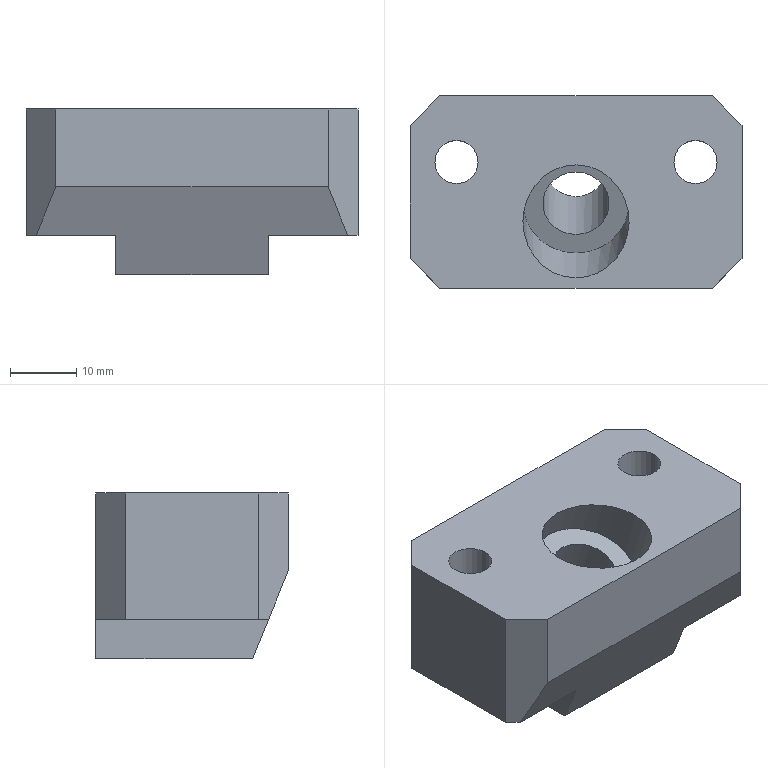Part | STEP file | lll_id298_x_t | 1 solid | 24 faces | box 50 x 29 x 25 mm | volume 24612 mm3 | plane 18 | cylinder 6 | commonest cylinder face diameters 6.5 x2 11 x2 10 x1 16 x1
STEP:
#1=CARTESIAN_POINT('',(0.,114.845,5.));
#2=VERTEX_POINT('',#1);
#3=CARTESIAN_POINT('',(0.,120.165,5.));
#4=DIRECTION('',(0.,0.,-1.));
#5=DIRECTION('',(0.,-1.,0.));
#6=AXIS2_PLACEMENT_3D('',#3,#4,#5);
#7=ELLIPSE('',#6,5.321,5.);
#8=EDGE_CURVE('',#2,#2,#7,.T.);
#9=ORIENTED_EDGE('',*,*,#8,.F.);
#10=EDGE_LOOP('',(#9));
#11=FACE_BOUND('',#10,.T.);
#12=CARTESIAN_POINT('',(-11.5,106.372,5.));
#13=VERTEX_POINT('',#12);
#14=CARTESIAN_POINT('',(11.5,106.372,5.));
#15=VERTEX_POINT('',#14);
#16=CARTESIAN_POINT('',(0.,106.372,5.));
#17=DIRECTION('',(1.,0.,0.));
#18=VECTOR('',#17,1.);
#19=LINE('',#16,#18);
#20=EDGE_CURVE('',#13,#15,#19,.T.);
#21=ORIENTED_EDGE('',*,*,#20,.F.);
#22=CARTESIAN_POINT('',(-11.5,130.,5.));
#23=VERTEX_POINT('',#22);
#24=CARTESIAN_POINT('',(-11.5,117.583,5.));
#25=DIRECTION('',(0.,-1.,0.));
#26=VECTOR('',#25,1.);
#27=LINE('',#24,#26);
#28=EDGE_CURVE('',#23,#13,#27,.T.);
#29=ORIENTED_EDGE('',*,*,#28,.F.);
#30=CARTESIAN_POINT('',(11.5,130.,5.));
#31=VERTEX_POINT('',#30);
#32=CARTESIAN_POINT('',(0.,130.,5.));
#33=DIRECTION('',(1.,0.,0.));
#34=VECTOR('',#33,1.);
#35=LINE('',#32,#34);
#36=EDGE_CURVE('',#23,#31,#35,.T.);
#37=ORIENTED_EDGE('',*,*,#36,.T.);
#38=CARTESIAN_POINT('',(11.5,117.583,5.));
#39=DIRECTION('',(0.,-1.,0.));
#40=VECTOR('',#39,1.);
#41=LINE('',#38,#40);
#42=EDGE_CURVE('',#31,#15,#41,.T.);
#43=ORIENTED_EDGE('',*,*,#42,.T.);
#44=EDGE_LOOP('',(#21,#29,#37,#43));
#45=FACE_BOUND('',#44,.T.);
#46=CARTESIAN_POINT('',(0.,116.372,5.));
#47=DIRECTION('',(0.,0.,-1.));
#48=DIRECTION('',(1.,0.,0.));
#49=AXIS2_PLACEMENT_3D('',#46,#47,#48);
#50=PLANE('',#49);
#51=ADVANCED_FACE('',(#11,#45),#50,.T.);
#52=CARTESIAN_POINT('',(-20.5,130.,11.));
#53=VERTEX_POINT('',#52);
#54=CARTESIAN_POINT('',(-11.5,130.,11.));
#55=VERTEX_POINT('',#54);
#56=CARTESIAN_POINT('',(0.,130.,11.));
#57=DIRECTION('',(1.,0.,0.));
#58=VECTOR('',#57,1.);
#59=LINE('',#56,#58);
#60=EDGE_CURVE('',#53,#55,#59,.T.);
#61=ORIENTED_EDGE('',*,*,#60,.F.);
#62=CARTESIAN_POINT('',(-20.5,130.,30.));
#63=VERTEX_POINT('',#62);
#64=CARTESIAN_POINT('',(-20.5,130.,-70.5));
#65=DIRECTION('',(0.,0.,1.));
#66=VECTOR('',#65,1.);
#67=LINE('',#64,#66);
#68=EDGE_CURVE('',#53,#63,#67,.T.);
#69=ORIENTED_EDGE('',*,*,#68,.T.);
#70=CARTESIAN_POINT('',(20.5,130.,30.));
#71=VERTEX_POINT('',#70);
#72=CARTESIAN_POINT('',(-0.004167,130.,30.));
#73=DIRECTION('',(1.,0.,0.));
#74=VECTOR('',#73,1.);
#75=LINE('',#72,#74);
#76=EDGE_CURVE('',#63,#71,#75,.T.);
#77=ORIENTED_EDGE('',*,*,#76,.T.);
#78=CARTESIAN_POINT('',(20.5,130.,11.));
#79=VERTEX_POINT('',#78);
#80=CARTESIAN_POINT('',(20.5,130.,11.));
#81=DIRECTION('',(0.,0.,-1.));
#82=VECTOR('',#81,1.);
#83=LINE('',#80,#82);
#84=EDGE_CURVE('',#71,#79,#83,.T.);
#85=ORIENTED_EDGE('',*,*,#84,.T.);
#86=CARTESIAN_POINT('',(11.5,130.,11.));
#87=VERTEX_POINT('',#86);
#88=CARTESIAN_POINT('',(0.,130.,11.));
#89=DIRECTION('',(1.,0.,0.));
#90=VECTOR('',#89,1.);
#91=LINE('',#88,#90);
#92=EDGE_CURVE('',#87,#79,#91,.T.);
#93=ORIENTED_EDGE('',*,*,#92,.F.);
#94=CARTESIAN_POINT('',(11.5,130.,2.003));
#95=DIRECTION('',(0.,0.,-1.));
#96=VECTOR('',#95,1.);
#97=LINE('',#94,#96);
#98=EDGE_CURVE('',#87,#31,#97,.T.);
#99=ORIENTED_EDGE('',*,*,#98,.T.);
#100=ORIENTED_EDGE('',*,*,#36,.F.);
#101=CARTESIAN_POINT('',(-11.5,130.,2.003));
#102=DIRECTION('',(0.,0.,-1.));
#103=VECTOR('',#102,1.);
#104=LINE('',#101,#103);
#105=EDGE_CURVE('',#55,#23,#104,.T.);
#106=ORIENTED_EDGE('',*,*,#105,.F.);
#107=EDGE_LOOP('',(#61,#69,#77,#85,#93,#99,#100,#106));
#108=FACE_OUTER_BOUND('',#107,.T.);
#109=CARTESIAN_POINT('',(0.,130.,-70.5));
#110=DIRECTION('',(0.,1.,0.));
#111=DIRECTION('',(0.,0.,1.));
#112=AXIS2_PLACEMENT_3D('',#109,#110,#111);
#113=PLANE('',#112);
#114=ADVANCED_FACE('',(#108),#113,.T.);
#115=CARTESIAN_POINT('',(20.5,101.,18.295));
#116=VERTEX_POINT('',#115);
#117=CARTESIAN_POINT('',(-20.5,101.,18.295));
#118=VERTEX_POINT('',#117);
#119=CARTESIAN_POINT('',(-0.004167,101.,18.295));
#120=DIRECTION('',(-1.,0.,0.));
#121=VECTOR('',#120,1.);
#122=LINE('',#119,#121);
#123=EDGE_CURVE('',#116,#118,#122,.T.);
#124=ORIENTED_EDGE('',*,*,#123,.T.);
#125=CARTESIAN_POINT('',(-23.448,103.948,11.));
#126=VERTEX_POINT('',#125);
#127=CARTESIAN_POINT('',(-18.043,98.543,24.378));
#128=DIRECTION('',(-0.3508,0.3508,-0.8683));
#129=VECTOR('',#128,1.);
#130=LINE('',#127,#129);
#131=EDGE_CURVE('',#118,#126,#130,.T.);
#132=ORIENTED_EDGE('',*,*,#131,.T.);
#133=CARTESIAN_POINT('',(-11.5,103.948,11.));
#134=VERTEX_POINT('',#133);
#135=CARTESIAN_POINT('',(-0.004167,103.948,11.));
#136=DIRECTION('',(1.,0.,0.));
#137=VECTOR('',#136,1.);
#138=LINE('',#135,#137);
#139=EDGE_CURVE('',#126,#134,#138,.T.);
#140=ORIENTED_EDGE('',*,*,#139,.T.);
#141=CARTESIAN_POINT('',(-11.5,108.986,-1.47));
#142=DIRECTION('',(0.,0.3746,-0.9272));
#143=VECTOR('',#142,1.);
#144=LINE('',#141,#143);
#145=EDGE_CURVE('',#134,#13,#144,.T.);
#146=ORIENTED_EDGE('',*,*,#145,.T.);
#147=ORIENTED_EDGE('',*,*,#20,.T.);
#148=CARTESIAN_POINT('',(11.5,103.948,11.));
#149=VERTEX_POINT('',#148);
#150=CARTESIAN_POINT('',(11.5,108.986,-1.47));
#151=DIRECTION('',(0.,0.3746,-0.9272));
#152=VECTOR('',#151,1.);
#153=LINE('',#150,#152);
#154=EDGE_CURVE('',#149,#15,#153,.T.);
#155=ORIENTED_EDGE('',*,*,#154,.F.);
#156=CARTESIAN_POINT('',(23.448,103.948,11.));
#157=VERTEX_POINT('',#156);
#158=CARTESIAN_POINT('',(-0.004167,103.948,11.));
#159=DIRECTION('',(1.,0.,0.));
#160=VECTOR('',#159,1.);
#161=LINE('',#158,#160);
#162=EDGE_CURVE('',#149,#157,#161,.T.);
#163=ORIENTED_EDGE('',*,*,#162,.T.);
#164=CARTESIAN_POINT('',(20.742,101.242,17.696));
#165=DIRECTION('',(-0.3508,-0.3508,0.8683));
#166=VECTOR('',#165,1.);
#167=LINE('',#164,#166);
#168=EDGE_CURVE('',#157,#116,#167,.T.);
#169=ORIENTED_EDGE('',*,*,#168,.T.);
#170=EDGE_LOOP('',(#124,#132,#140,#146,#147,#155,#163,#169));
#171=FACE_OUTER_BOUND('',#170,.T.);
#172=CARTESIAN_POINT('',(-0.004167,107.583,2.003));
#173=DIRECTION('',(0.,0.9272,0.3746));
#174=DIRECTION('',(0.,-0.3746,0.9272));
#175=AXIS2_PLACEMENT_3D('',#172,#173,#174);
#176=PLANE('',#175);
#177=ADVANCED_FACE('',(#171),#176,.F.);
#178=CARTESIAN_POINT('',(11.5,117.583,11.));
#179=DIRECTION('',(0.,1.,0.));
#180=VECTOR('',#179,1.);
#181=LINE('',#178,#180);
#182=EDGE_CURVE('',#149,#87,#181,.T.);
#183=ORIENTED_EDGE('',*,*,#182,.F.);
#184=ORIENTED_EDGE('',*,*,#154,.T.);
#185=ORIENTED_EDGE('',*,*,#42,.F.);
#186=ORIENTED_EDGE('',*,*,#98,.F.);
#187=EDGE_LOOP('',(#183,#184,#185,#186));
#188=FACE_OUTER_BOUND('',#187,.T.);
#189=CARTESIAN_POINT('',(11.5,117.583,2.003));
#190=DIRECTION('',(-1.,0.,0.));
#191=DIRECTION('',(0.,0.,-1.));
#192=AXIS2_PLACEMENT_3D('',#189,#190,#191);
#193=PLANE('',#192);
#194=ADVANCED_FACE('',(#188),#193,.F.);
#195=ORIENTED_EDGE('',*,*,#145,.F.);
#196=CARTESIAN_POINT('',(-11.5,117.583,11.));
#197=DIRECTION('',(0.,1.,0.));
#198=VECTOR('',#197,1.);
#199=LINE('',#196,#198);
#200=EDGE_CURVE('',#134,#55,#199,.T.);
#201=ORIENTED_EDGE('',*,*,#200,.T.);
#202=ORIENTED_EDGE('',*,*,#105,.T.);
#203=ORIENTED_EDGE('',*,*,#28,.T.);
#204=EDGE_LOOP('',(#195,#201,#202,#203));
#205=FACE_OUTER_BOUND('',#204,.T.);
#206=CARTESIAN_POINT('',(-11.5,117.583,2.003));
#207=DIRECTION('',(-1.,0.,0.));
#208=DIRECTION('',(0.,0.,-1.));
#209=AXIS2_PLACEMENT_3D('',#206,#207,#208);
#210=PLANE('',#209);
#211=ADVANCED_FACE('',(#205),#210,.T.);
#212=CARTESIAN_POINT('',(12.5,120.,11.));
#213=VERTEX_POINT('',#212);
#214=CARTESIAN_POINT('',(18.,120.,11.));
#215=DIRECTION('',(0.,0.,1.));
#216=DIRECTION('',(-1.,0.,0.));
#217=AXIS2_PLACEMENT_3D('',#214,#215,#216);
#218=CIRCLE('',#217,5.5);
#219=EDGE_CURVE('',#213,#213,#218,.T.);
#220=ORIENTED_EDGE('',*,*,#219,.T.);
#221=EDGE_LOOP('',(#220));
#222=FACE_BOUND('',#221,.T.);
#223=ORIENTED_EDGE('',*,*,#92,.T.);
#224=CARTESIAN_POINT('',(25.,125.5,11.));
#225=VERTEX_POINT('',#224);
#226=CARTESIAN_POINT('',(20.5,130.,11.));
#227=DIRECTION('',(0.7071,-0.7071,0.));
#228=VECTOR('',#227,1.);
#229=LINE('',#226,#228);
#230=EDGE_CURVE('',#79,#225,#229,.T.);
#231=ORIENTED_EDGE('',*,*,#230,.T.);
#232=CARTESIAN_POINT('',(25.,105.5,11.));
#233=VERTEX_POINT('',#232);
#234=CARTESIAN_POINT('',(25.,110.311,11.));
#235=DIRECTION('',(0.,1.,0.));
#236=VECTOR('',#235,1.);
#237=LINE('',#234,#236);
#238=EDGE_CURVE('',#233,#225,#237,.T.);
#239=ORIENTED_EDGE('',*,*,#238,.F.);
#240=CARTESIAN_POINT('',(20.5,101.,11.));
#241=DIRECTION('',(-0.7071,-0.7071,0.));
#242=VECTOR('',#241,1.);
#243=LINE('',#240,#242);
#244=EDGE_CURVE('',#233,#157,#243,.T.);
#245=ORIENTED_EDGE('',*,*,#244,.T.);
#246=ORIENTED_EDGE('',*,*,#162,.F.);
#247=ORIENTED_EDGE('',*,*,#182,.T.);
#248=EDGE_LOOP('',(#223,#231,#239,#245,#246,#247));
#249=FACE_BOUND('',#248,.T.);
#250=CARTESIAN_POINT('',(20.5,115.,11.));
#251=DIRECTION('',(0.,0.,1.));
#252=DIRECTION('',(-1.,0.,0.));
#253=AXIS2_PLACEMENT_3D('',#250,#251,#252);
#254=PLANE('',#253);
#255=ADVANCED_FACE('',(#222,#249),#254,.F.);
#256=CARTESIAN_POINT('',(-25.,105.5,11.));
#257=VERTEX_POINT('',#256);
#258=CARTESIAN_POINT('',(-25.,125.5,11.));
#259=VERTEX_POINT('',#258);
#260=CARTESIAN_POINT('',(-25.,110.311,11.));
#261=DIRECTION('',(0.,1.,0.));
#262=VECTOR('',#261,1.);
#263=LINE('',#260,#262);
#264=EDGE_CURVE('',#257,#259,#263,.T.);
#265=ORIENTED_EDGE('',*,*,#264,.F.);
#266=CARTESIAN_POINT('',(-25.,105.5,30.));
#267=VERTEX_POINT('',#266);
#268=CARTESIAN_POINT('',(-25.,105.5,30.));
#269=DIRECTION('',(0.,0.,1.));
#270=VECTOR('',#269,1.);
#271=LINE('',#268,#270);
#272=EDGE_CURVE('',#257,#267,#271,.T.);
#273=ORIENTED_EDGE('',*,*,#272,.T.);
#274=CARTESIAN_POINT('',(-25.,125.5,30.));
#275=VERTEX_POINT('',#274);
#276=CARTESIAN_POINT('',(-25.,110.311,30.));
#277=DIRECTION('',(0.,-1.,0.));
#278=VECTOR('',#277,1.);
#279=LINE('',#276,#278);
#280=EDGE_CURVE('',#275,#267,#279,.T.);
#281=ORIENTED_EDGE('',*,*,#280,.F.);
#282=CARTESIAN_POINT('',(-25.,125.5,30.));
#283=DIRECTION('',(0.,0.,-1.));
#284=VECTOR('',#283,1.);
#285=LINE('',#282,#284);
#286=EDGE_CURVE('',#275,#259,#285,.T.);
#287=ORIENTED_EDGE('',*,*,#286,.T.);
#288=EDGE_LOOP('',(#265,#273,#281,#287));
#289=FACE_OUTER_BOUND('',#288,.T.);
#290=CARTESIAN_POINT('',(-25.,110.311,30.));
#291=DIRECTION('',(1.,0.,0.));
#292=DIRECTION('',(0.,0.,1.));
#293=AXIS2_PLACEMENT_3D('',#290,#291,#292);
#294=PLANE('',#293);
#295=ADVANCED_FACE('',(#289),#294,.F.);
#296=ORIENTED_EDGE('',*,*,#238,.T.);
#297=CARTESIAN_POINT('',(25.,125.5,30.));
#298=VERTEX_POINT('',#297);
#299=CARTESIAN_POINT('',(25.,125.5,30.));
#300=DIRECTION('',(0.,0.,1.));
#301=VECTOR('',#300,1.);
#302=LINE('',#299,#301);
#303=EDGE_CURVE('',#225,#298,#302,.T.);
#304=ORIENTED_EDGE('',*,*,#303,.T.);
#305=CARTESIAN_POINT('',(25.,105.5,30.));
#306=VERTEX_POINT('',#305);
#307=CARTESIAN_POINT('',(25.,110.311,30.));
#308=DIRECTION('',(0.,-1.,0.));
#309=VECTOR('',#308,1.);
#310=LINE('',#307,#309);
#311=EDGE_CURVE('',#298,#306,#310,.T.);
#312=ORIENTED_EDGE('',*,*,#311,.T.);
#313=CARTESIAN_POINT('',(25.,105.5,30.));
#314=DIRECTION('',(0.,0.,-1.));
#315=VECTOR('',#314,1.);
#316=LINE('',#313,#315);
#317=EDGE_CURVE('',#306,#233,#316,.T.);
#318=ORIENTED_EDGE('',*,*,#317,.T.);
#319=EDGE_LOOP('',(#296,#304,#312,#318));
#320=FACE_OUTER_BOUND('',#319,.T.);
#321=CARTESIAN_POINT('',(25.,110.311,30.));
#322=DIRECTION('',(1.,0.,0.));
#323=DIRECTION('',(0.,0.,1.));
#324=AXIS2_PLACEMENT_3D('',#321,#322,#323);
#325=PLANE('',#324);
#326=ADVANCED_FACE('',(#320),#325,.T.);
#327=CARTESIAN_POINT('',(0.,102.553,30.));
#328=VERTEX_POINT('',#327);
#329=CARTESIAN_POINT('',(0.,111.066,30.));
#330=DIRECTION('',(0.,0.,-1.));
#331=DIRECTION('',(0.,-1.,0.));
#332=AXIS2_PLACEMENT_3D('',#329,#330,#331);
#333=ELLIPSE('',#332,8.513,8.);
#334=EDGE_CURVE('',#328,#328,#333,.T.);
#335=ORIENTED_EDGE('',*,*,#334,.T.);
#336=EDGE_LOOP('',(#335));
#337=FACE_BOUND('',#336,.T.);
#338=CARTESIAN_POINT('',(-14.75,120.,30.));
#339=VERTEX_POINT('',#338);
#340=CARTESIAN_POINT('',(-18.,120.,30.));
#341=DIRECTION('',(0.,0.,-1.));
#342=DIRECTION('',(1.,0.,0.));
#343=AXIS2_PLACEMENT_3D('',#340,#341,#342);
#344=CIRCLE('',#343,3.25);
#345=EDGE_CURVE('',#339,#339,#344,.T.);
#346=ORIENTED_EDGE('',*,*,#345,.T.);
#347=EDGE_LOOP('',(#346));
#348=FACE_BOUND('',#347,.T.);
#349=CARTESIAN_POINT('',(21.25,120.,30.));
#350=VERTEX_POINT('',#349);
#351=CARTESIAN_POINT('',(18.,120.,30.));
#352=DIRECTION('',(0.,0.,-1.));
#353=DIRECTION('',(1.,0.,0.));
#354=AXIS2_PLACEMENT_3D('',#351,#352,#353);
#355=CIRCLE('',#354,3.25);
#356=EDGE_CURVE('',#350,#350,#355,.T.);
#357=ORIENTED_EDGE('',*,*,#356,.T.);
#358=EDGE_LOOP('',(#357));
#359=FACE_BOUND('',#358,.T.);
#360=ORIENTED_EDGE('',*,*,#280,.T.);
#361=CARTESIAN_POINT('',(-20.5,101.,30.));
#362=VERTEX_POINT('',#361);
#363=CARTESIAN_POINT('',(-25.,105.5,30.));
#364=DIRECTION('',(0.7071,-0.7071,0.));
#365=VECTOR('',#364,1.);
#366=LINE('',#363,#365);
#367=EDGE_CURVE('',#267,#362,#366,.T.);
#368=ORIENTED_EDGE('',*,*,#367,.T.);
#369=CARTESIAN_POINT('',(20.5,101.,30.));
#370=VERTEX_POINT('',#369);
#371=CARTESIAN_POINT('',(-0.004167,101.,30.));
#372=DIRECTION('',(1.,0.,0.));
#373=VECTOR('',#372,1.);
#374=LINE('',#371,#373);
#375=EDGE_CURVE('',#362,#370,#374,.T.);
#376=ORIENTED_EDGE('',*,*,#375,.T.);
#377=CARTESIAN_POINT('',(20.5,101.,30.));
#378=DIRECTION('',(0.7071,0.7071,0.));
#379=VECTOR('',#378,1.);
#380=LINE('',#377,#379);
#381=EDGE_CURVE('',#370,#306,#380,.T.);
#382=ORIENTED_EDGE('',*,*,#381,.T.);
#383=ORIENTED_EDGE('',*,*,#311,.F.);
#384=CARTESIAN_POINT('',(20.5,130.,30.));
#385=DIRECTION('',(-0.7071,0.7071,0.));
#386=VECTOR('',#385,1.);
#387=LINE('',#384,#386);
#388=EDGE_CURVE('',#298,#71,#387,.T.);
#389=ORIENTED_EDGE('',*,*,#388,.T.);
#390=ORIENTED_EDGE('',*,*,#76,.F.);
#391=CARTESIAN_POINT('',(-25.,125.5,30.));
#392=DIRECTION('',(-0.7071,-0.7071,0.));
#393=VECTOR('',#392,1.);
#394=LINE('',#391,#393);
#395=EDGE_CURVE('',#63,#275,#394,.T.);
#396=ORIENTED_EDGE('',*,*,#395,.T.);
#397=EDGE_LOOP('',(#360,#368,#376,#382,#383,#389,#390,#396));
#398=FACE_BOUND('',#397,.T.);
#399=CARTESIAN_POINT('',(-0.004167,110.311,30.));
#400=DIRECTION('',(0.,0.,-1.));
#401=DIRECTION('',(1.,0.,0.));
#402=AXIS2_PLACEMENT_3D('',#399,#400,#401);
#403=PLANE('',#402);
#404=ADVANCED_FACE('',(#337,#348,#359,#398),#403,.F.);
#405=ORIENTED_EDGE('',*,*,#375,.F.);
#406=CARTESIAN_POINT('',(-20.5,101.,18.295));
#407=DIRECTION('',(0.,0.,-1.));
#408=VECTOR('',#407,1.);
#409=LINE('',#406,#408);
#410=EDGE_CURVE('',#362,#118,#409,.T.);
#411=ORIENTED_EDGE('',*,*,#410,.T.);
#412=ORIENTED_EDGE('',*,*,#123,.F.);
#413=CARTESIAN_POINT('',(20.5,101.,17.5));
#414=DIRECTION('',(0.,0.,1.));
#415=VECTOR('',#414,1.);
#416=LINE('',#413,#415);
#417=EDGE_CURVE('',#116,#370,#416,.T.);
#418=ORIENTED_EDGE('',*,*,#417,.T.);
#419=EDGE_LOOP('',(#405,#411,#412,#418));
#420=FACE_OUTER_BOUND('',#419,.T.);
#421=CARTESIAN_POINT('',(0.,101.,17.5));
#422=DIRECTION('',(0.,1.,0.));
#423=DIRECTION('',(0.,0.,-1.));
#424=AXIS2_PLACEMENT_3D('',#421,#422,#423);
#425=PLANE('',#424);
#426=ADVANCED_FACE('',(#420),#425,.F.);
#427=CARTESIAN_POINT('',(-12.5,120.,11.));
#428=VERTEX_POINT('',#427);
#429=CARTESIAN_POINT('',(-18.,120.,11.));
#430=DIRECTION('',(0.,0.,-1.));
#431=DIRECTION('',(1.,0.,0.));
#432=AXIS2_PLACEMENT_3D('',#429,#430,#431);
#433=CIRCLE('',#432,5.5);
#434=EDGE_CURVE('',#428,#428,#433,.T.);
#435=ORIENTED_EDGE('',*,*,#434,.F.);
#436=EDGE_LOOP('',(#435));
#437=FACE_BOUND('',#436,.T.);
#438=ORIENTED_EDGE('',*,*,#139,.F.);
#439=CARTESIAN_POINT('',(-25.,105.5,11.));
#440=DIRECTION('',(-0.7071,0.7071,0.));
#441=VECTOR('',#440,1.);
#442=LINE('',#439,#441);
#443=EDGE_CURVE('',#126,#257,#442,.T.);
#444=ORIENTED_EDGE('',*,*,#443,.T.);
#445=ORIENTED_EDGE('',*,*,#264,.T.);
#446=CARTESIAN_POINT('',(-25.,125.5,11.));
#447=DIRECTION('',(0.7071,0.7071,0.));
#448=VECTOR('',#447,1.);
#449=LINE('',#446,#448);
#450=EDGE_CURVE('',#259,#53,#449,.T.);
#451=ORIENTED_EDGE('',*,*,#450,.T.);
#452=ORIENTED_EDGE('',*,*,#60,.T.);
#453=ORIENTED_EDGE('',*,*,#200,.F.);
#454=EDGE_LOOP('',(#438,#444,#445,#451,#452,#453));
#455=FACE_BOUND('',#454,.T.);
#456=CARTESIAN_POINT('',(20.5,115.,11.));
#457=DIRECTION('',(0.,0.,1.));
#458=DIRECTION('',(-1.,0.,0.));
#459=AXIS2_PLACEMENT_3D('',#456,#457,#458);
#460=PLANE('',#459);
#461=ADVANCED_FACE('',(#437,#455),#460,.F.);
#462=CARTESIAN_POINT('',(14.75,120.,17.5));
#463=VERTEX_POINT('',#462);
#464=CARTESIAN_POINT('',(18.,120.,17.5));
#465=DIRECTION('',(0.,0.,1.));
#466=DIRECTION('',(-1.,0.,0.));
#467=AXIS2_PLACEMENT_3D('',#464,#465,#466);
#468=CIRCLE('',#467,3.25);
#469=EDGE_CURVE('',#463,#463,#468,.T.);
#470=ORIENTED_EDGE('',*,*,#469,.F.);
#471=EDGE_LOOP('',(#470));
#472=FACE_BOUND('',#471,.T.);
#473=ORIENTED_EDGE('',*,*,#356,.F.);
#474=EDGE_LOOP('',(#473));
#475=FACE_BOUND('',#474,.T.);
#476=CARTESIAN_POINT('',(18.,120.,311.));
#477=DIRECTION('',(0.,0.,1.));
#478=DIRECTION('',(-1.,0.,0.));
#479=AXIS2_PLACEMENT_3D('',#476,#477,#478);
#480=CYLINDRICAL_SURFACE('',#479,3.25);
#481=ADVANCED_FACE('',(#472,#475),#480,.F.);
#482=ORIENTED_EDGE('',*,*,#469,.T.);
#483=EDGE_LOOP('',(#482));
#484=FACE_BOUND('',#483,.T.);
#485=CARTESIAN_POINT('',(12.5,120.,17.5));
#486=VERTEX_POINT('',#485);
#487=CARTESIAN_POINT('',(18.,120.,17.5));
#488=DIRECTION('',(0.,0.,1.));
#489=DIRECTION('',(-1.,0.,0.));
#490=AXIS2_PLACEMENT_3D('',#487,#488,#489);
#491=CIRCLE('',#490,5.5);
#492=EDGE_CURVE('',#486,#486,#491,.T.);
#493=ORIENTED_EDGE('',*,*,#492,.F.);
#494=EDGE_LOOP('',(#493));
#495=FACE_BOUND('',#494,.T.);
#496=CARTESIAN_POINT('',(18.,120.,17.5));
#497=DIRECTION('',(0.,0.,1.));
#498=DIRECTION('',(-1.,0.,0.));
#499=AXIS2_PLACEMENT_3D('',#496,#497,#498);
#500=PLANE('',#499);
#501=ADVANCED_FACE('',(#484,#495),#500,.F.);
#502=ORIENTED_EDGE('',*,*,#492,.T.);
#503=EDGE_LOOP('',(#502));
#504=FACE_BOUND('',#503,.T.);
#505=ORIENTED_EDGE('',*,*,#219,.F.);
#506=EDGE_LOOP('',(#505));
#507=FACE_BOUND('',#506,.T.);
#508=CARTESIAN_POINT('',(18.,120.,11.));
#509=DIRECTION('',(0.,0.,1.));
#510=DIRECTION('',(-1.,0.,0.));
#511=AXIS2_PLACEMENT_3D('',#508,#509,#510);
#512=CYLINDRICAL_SURFACE('',#511,5.5);
#513=ADVANCED_FACE('',(#504,#507),#512,.F.);
#514=CARTESIAN_POINT('',(-14.75,120.,17.5));
#515=VERTEX_POINT('',#514);
#516=CARTESIAN_POINT('',(-18.,120.,17.5));
#517=DIRECTION('',(0.,0.,-1.));
#518=DIRECTION('',(1.,0.,0.));
#519=AXIS2_PLACEMENT_3D('',#516,#517,#518);
#520=CIRCLE('',#519,3.25);
#521=EDGE_CURVE('',#515,#515,#520,.T.);
#522=ORIENTED_EDGE('',*,*,#521,.T.);
#523=EDGE_LOOP('',(#522));
#524=FACE_BOUND('',#523,.T.);
#525=ORIENTED_EDGE('',*,*,#345,.F.);
#526=EDGE_LOOP('',(#525));
#527=FACE_BOUND('',#526,.T.);
#528=CARTESIAN_POINT('',(-18.,120.,311.));
#529=DIRECTION('',(0.,0.,1.));
#530=DIRECTION('',(1.,0.,0.));
#531=AXIS2_PLACEMENT_3D('',#528,#529,#530);
#532=CYLINDRICAL_SURFACE('',#531,3.25);
#533=ADVANCED_FACE('',(#524,#527),#532,.F.);
#534=ORIENTED_EDGE('',*,*,#521,.F.);
#535=EDGE_LOOP('',(#534));
#536=FACE_BOUND('',#535,.T.);
#537=CARTESIAN_POINT('',(-12.5,120.,17.5));
#538=VERTEX_POINT('',#537);
#539=CARTESIAN_POINT('',(-18.,120.,17.5));
#540=DIRECTION('',(0.,0.,-1.));
#541=DIRECTION('',(1.,0.,0.));
#542=AXIS2_PLACEMENT_3D('',#539,#540,#541);
#543=CIRCLE('',#542,5.5);
#544=EDGE_CURVE('',#538,#538,#543,.T.);
#545=ORIENTED_EDGE('',*,*,#544,.T.);
#546=EDGE_LOOP('',(#545));
#547=FACE_BOUND('',#546,.T.);
#548=CARTESIAN_POINT('',(-18.,120.,17.5));
#549=DIRECTION('',(0.,0.,1.));
#550=DIRECTION('',(1.,0.,0.));
#551=AXIS2_PLACEMENT_3D('',#548,#549,#550);
#552=PLANE('',#551);
#553=ADVANCED_FACE('',(#536,#547),#552,.F.);
#554=ORIENTED_EDGE('',*,*,#544,.F.);
#555=EDGE_LOOP('',(#554));
#556=FACE_BOUND('',#555,.T.);
#557=ORIENTED_EDGE('',*,*,#434,.T.);
#558=EDGE_LOOP('',(#557));
#559=FACE_BOUND('',#558,.T.);
#560=CARTESIAN_POINT('',(-18.,120.,11.));
#561=DIRECTION('',(0.,0.,1.));
#562=DIRECTION('',(1.,0.,0.));
#563=AXIS2_PLACEMENT_3D('',#560,#561,#562);
#564=CYLINDRICAL_SURFACE('',#563,5.5);
#565=ADVANCED_FACE('',(#556,#559),#564,.F.);
#566=CARTESIAN_POINT('',(0.,106.285,19.746));
#567=VERTEX_POINT('',#566);
#568=CARTESIAN_POINT('',(0.,113.802,22.482));
#569=DIRECTION('',(0.,-0.342,0.9397));
#570=DIRECTION('',(0.,-0.9397,-0.342));
#571=AXIS2_PLACEMENT_3D('',#568,#569,#570);
#572=CIRCLE('',#571,8.);
#573=EDGE_CURVE('',#567,#567,#572,.T.);
#574=ORIENTED_EDGE('',*,*,#573,.F.);
#575=EDGE_LOOP('',(#574));
#576=FACE_BOUND('',#575,.T.);
#577=ORIENTED_EDGE('',*,*,#334,.F.);
#578=EDGE_LOOP('',(#577));
#579=FACE_BOUND('',#578,.T.);
#580=CARTESIAN_POINT('',(0.,113.802,22.482));
#581=DIRECTION('',(0.,-0.342,0.9397));
#582=DIRECTION('',(0.,0.9397,0.342));
#583=AXIS2_PLACEMENT_3D('',#580,#581,#582);
#584=CYLINDRICAL_SURFACE('',#583,8.);
#585=ADVANCED_FACE('',(#576,#579),#584,.F.);
#586=ORIENTED_EDGE('',*,*,#8,.T.);
#587=EDGE_LOOP('',(#586));
#588=FACE_BOUND('',#587,.T.);
#589=CARTESIAN_POINT('',(0.,109.104,20.772));
#590=VERTEX_POINT('',#589);
#591=CARTESIAN_POINT('',(0.,113.802,22.482));
#592=DIRECTION('',(0.,-0.342,0.9397));
#593=DIRECTION('',(0.,-0.9397,-0.342));
#594=AXIS2_PLACEMENT_3D('',#591,#592,#593);
#595=CIRCLE('',#594,5.);
#596=EDGE_CURVE('',#590,#590,#595,.T.);
#597=ORIENTED_EDGE('',*,*,#596,.T.);
#598=EDGE_LOOP('',(#597));
#599=FACE_BOUND('',#598,.T.);
#600=CARTESIAN_POINT('',(0.,138.,-44.));
#601=DIRECTION('',(0.,-0.342,0.9397));
#602=DIRECTION('',(-1.,0.,0.));
#603=AXIS2_PLACEMENT_3D('',#600,#601,#602);
#604=CYLINDRICAL_SURFACE('',#603,5.);
#605=ADVANCED_FACE('',(#588,#599),#604,.F.);
#606=ORIENTED_EDGE('',*,*,#596,.F.);
#607=EDGE_LOOP('',(#606));
#608=FACE_BOUND('',#607,.T.);
#609=ORIENTED_EDGE('',*,*,#573,.T.);
#610=EDGE_LOOP('',(#609));
#611=FACE_BOUND('',#610,.T.);
#612=CARTESIAN_POINT('',(0.,113.802,22.482));
#613=DIRECTION('',(0.,0.342,-0.9397));
#614=DIRECTION('',(0.,-0.9397,-0.342));
#615=AXIS2_PLACEMENT_3D('',#612,#613,#614);
#616=PLANE('',#615);
#617=ADVANCED_FACE('',(#608,#611),#616,.F.);
#618=ORIENTED_EDGE('',*,*,#131,.F.);
#619=ORIENTED_EDGE('',*,*,#410,.F.);
#620=ORIENTED_EDGE('',*,*,#367,.F.);
#621=ORIENTED_EDGE('',*,*,#272,.F.);
#622=ORIENTED_EDGE('',*,*,#443,.F.);
#623=EDGE_LOOP('',(#618,#619,#620,#621,#622));
#624=FACE_OUTER_BOUND('',#623,.T.);
#625=CARTESIAN_POINT('',(-25.,105.5,30.));
#626=DIRECTION('',(0.7071,0.7071,0.));
#627=DIRECTION('',(-0.7071,0.7071,0.));
#628=AXIS2_PLACEMENT_3D('',#625,#626,#627);
#629=PLANE('',#628);
#630=ADVANCED_FACE('',(#624),#629,.F.);
#631=ORIENTED_EDGE('',*,*,#395,.F.);
#632=ORIENTED_EDGE('',*,*,#68,.F.);
#633=ORIENTED_EDGE('',*,*,#450,.F.);
#634=ORIENTED_EDGE('',*,*,#286,.F.);
#635=EDGE_LOOP('',(#631,#632,#633,#634));
#636=FACE_OUTER_BOUND('',#635,.T.);
#637=CARTESIAN_POINT('',(-25.,125.5,30.));
#638=DIRECTION('',(-0.7071,0.7071,0.));
#639=DIRECTION('',(-0.7071,-0.7071,0.));
#640=AXIS2_PLACEMENT_3D('',#637,#638,#639);
#641=PLANE('',#640);
#642=ADVANCED_FACE('',(#636),#641,.T.);
#643=ORIENTED_EDGE('',*,*,#388,.F.);
#644=ORIENTED_EDGE('',*,*,#303,.F.);
#645=ORIENTED_EDGE('',*,*,#230,.F.);
#646=ORIENTED_EDGE('',*,*,#84,.F.);
#647=EDGE_LOOP('',(#643,#644,#645,#646));
#648=FACE_OUTER_BOUND('',#647,.T.);
#649=CARTESIAN_POINT('',(20.5,130.,-70.5));
#650=DIRECTION('',(-0.7071,-0.7071,0.));
#651=DIRECTION('',(0.7071,-0.7071,0.));
#652=AXIS2_PLACEMENT_3D('',#649,#650,#651);
#653=PLANE('',#652);
#654=ADVANCED_FACE('',(#648),#653,.F.);
#655=ORIENTED_EDGE('',*,*,#244,.F.);
#656=ORIENTED_EDGE('',*,*,#317,.F.);
#657=ORIENTED_EDGE('',*,*,#381,.F.);
#658=ORIENTED_EDGE('',*,*,#417,.F.);
#659=ORIENTED_EDGE('',*,*,#168,.F.);
#660=EDGE_LOOP('',(#655,#656,#657,#658,#659));
#661=FACE_OUTER_BOUND('',#660,.T.);
#662=CARTESIAN_POINT('',(20.5,101.,17.5));
#663=DIRECTION('',(0.7071,-0.7071,0.));
#664=DIRECTION('',(0.7071,0.7071,0.));
#665=AXIS2_PLACEMENT_3D('',#662,#663,#664);
#666=PLANE('',#665);
#667=ADVANCED_FACE('',(#661),#666,.T.);
#668=CLOSED_SHELL('',(#51,#114,#177,#194,#211,#255,#295,#326,#404,#426,#461,#481,#501,#513,#533,#553,#565,#585,#605,#617,#630,#642,#654,#667));
#669=MANIFOLD_SOLID_BREP('',#668);
#670=(LENGTH_UNIT()NAMED_UNIT(*)SI_UNIT(.MILLI.,.METRE.));
#671=UNCERTAINTY_MEASURE_WITH_UNIT(LENGTH_MEASURE(0.00002),#670,'','');
#672=(NAMED_UNIT(*)PLANE_ANGLE_UNIT()SI_UNIT($,.RADIAN.));
#673=PLANE_ANGLE_MEASURE_WITH_UNIT(PLANE_ANGLE_MEASURE(0.01745),#672);
#674=DIMENSIONAL_EXPONENTS(0.,0.,0.,0.,0.,0.,0.);
#675=(CONVERSION_BASED_UNIT('DEGREE',#673)NAMED_UNIT(#674)PLANE_ANGLE_UNIT());
#676=(NAMED_UNIT(*)SI_UNIT($,.STERADIAN.)SOLID_ANGLE_UNIT());
#677=(GEOMETRIC_REPRESENTATION_CONTEXT(3)GLOBAL_UNCERTAINTY_ASSIGNED_CONTEXT((#671))GLOBAL_UNIT_ASSIGNED_CONTEXT((#670,#675,#676))REPRESENTATION_CONTEXT('',''));
#678=ADVANCED_BREP_SHAPE_REPRESENTATION('',(#669),#677);